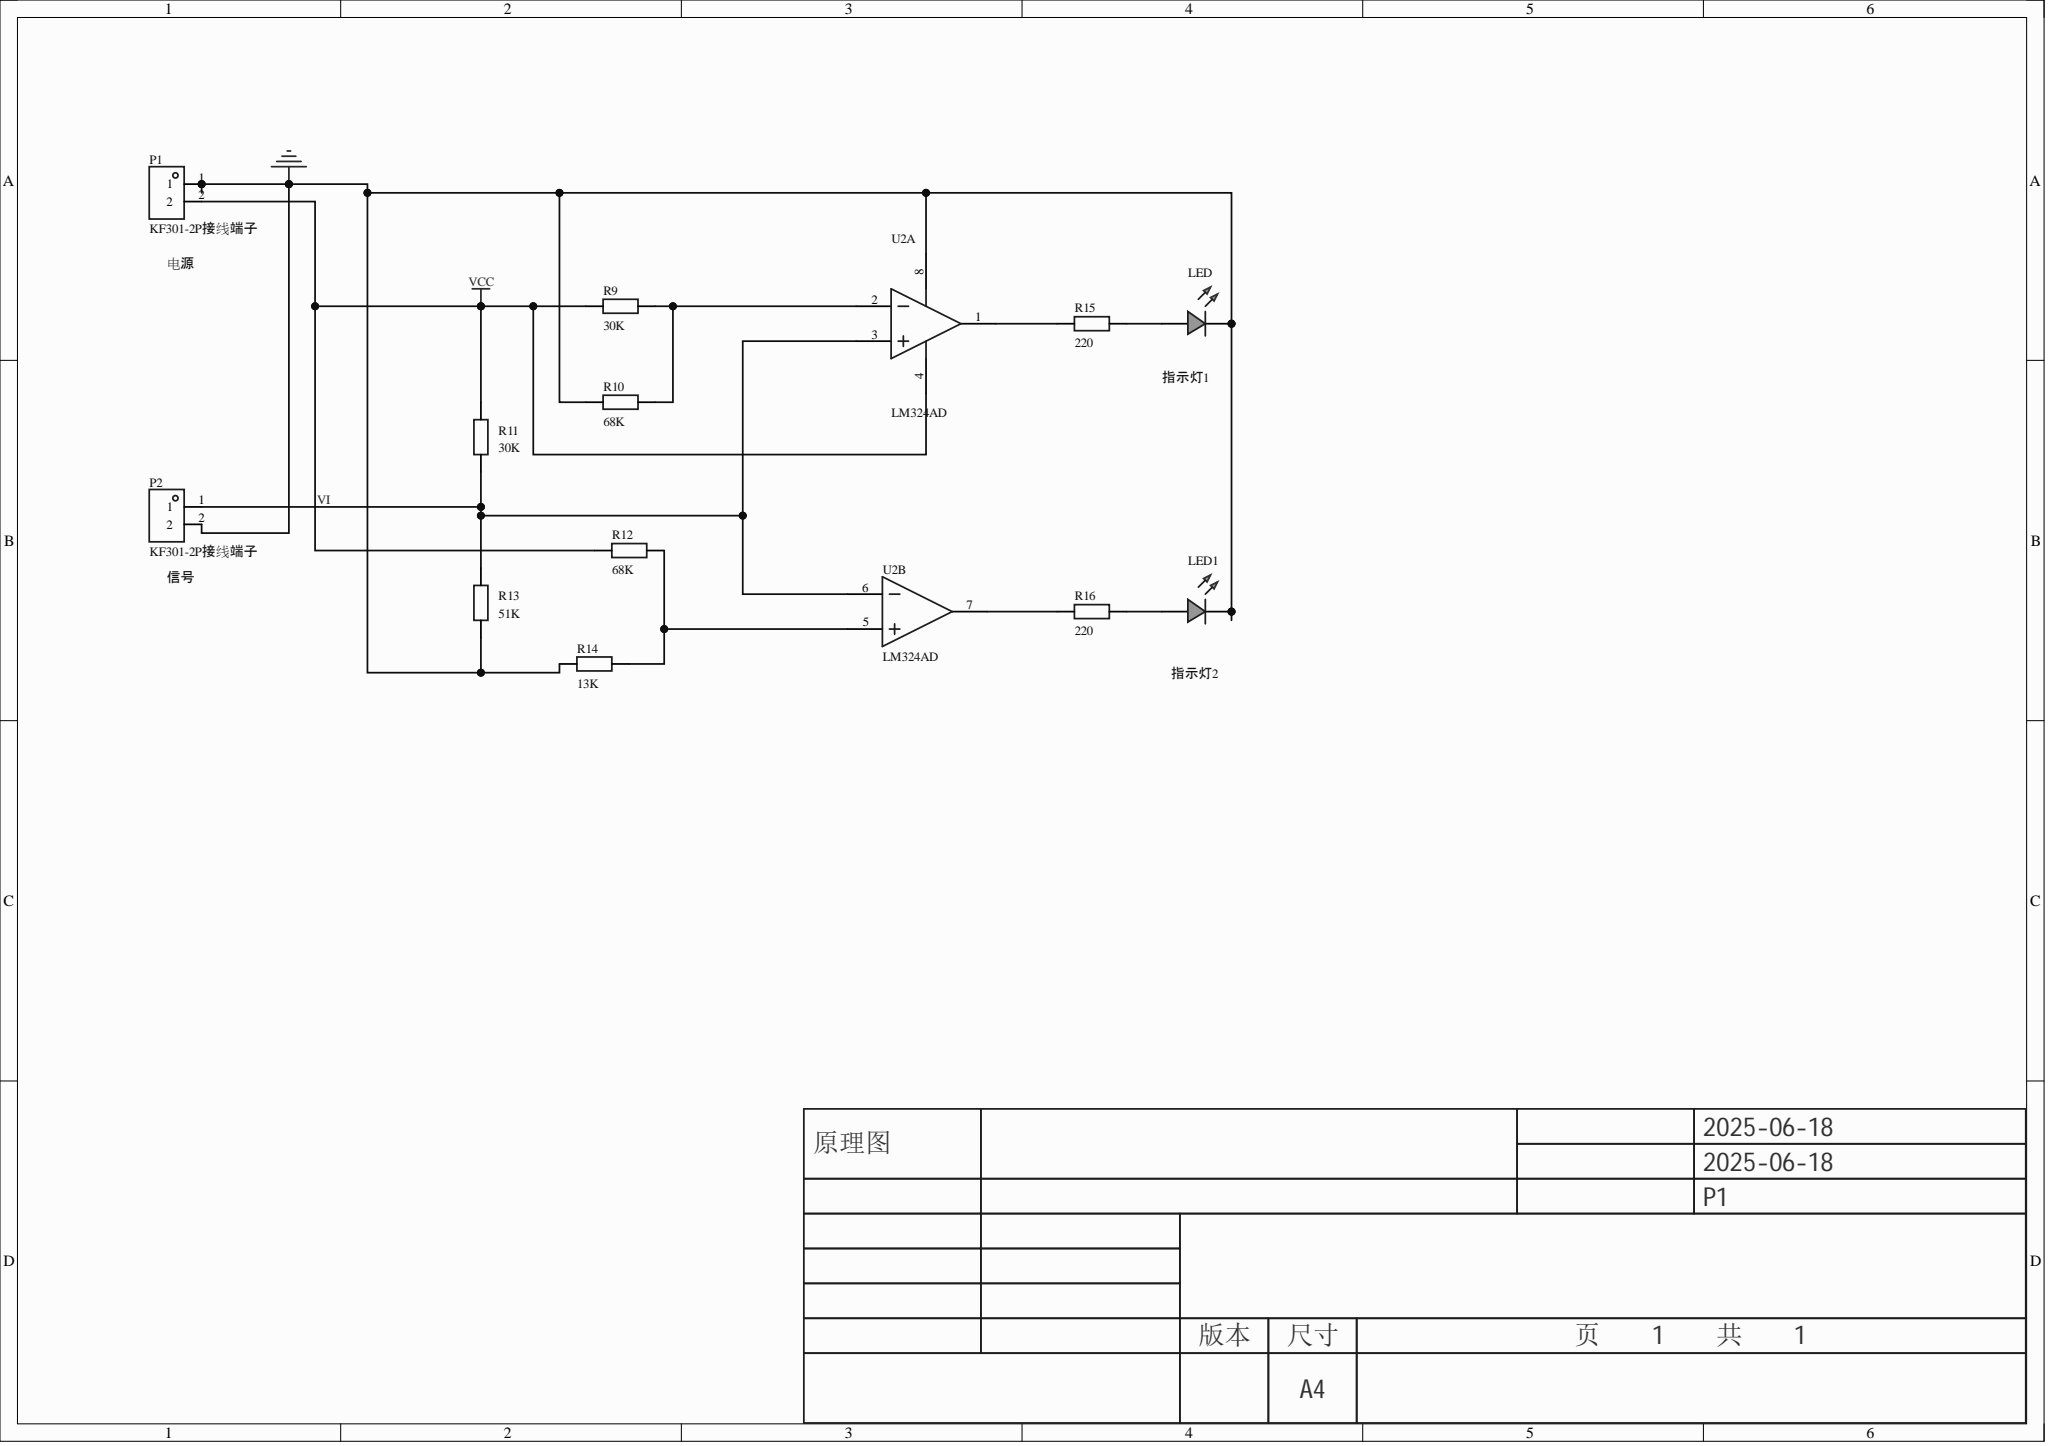Circuit board | Altium Designer | 13 parts | 9 nets
Bill of materials:
Comment,Description,Designator,Footprint,LibRef,Quantity
"","","LED, LED1","LED-TH_5mm","LED_TH-G_5mm","2"
"KF301-2P接线端子","","P1, P2","CONN-TH_XY301V-A-5.0-2P","KF301-2P接线端子","2"
"30K","","R9, R11","Res_1/8W","Res_AXIAL-1/8W","2"
"68K","","R10, R12","Res_1/8W","Res_AXIAL-1/8W","2"
"51K","","R13","Res_1/8W","Res_AXIAL-1/8W","1"
"13K","","R14","Res_1/8W","Res_AXIAL-1/8W","1"
"220","","R15, R16","Res_1/8W","Res_AXIAL-1/8W","2"
"LM324AD","放大器数:双路;轨到轨:-;增益带宽积(GBP):10MHz;输入失调电压(Vos):5mV;压摆率(SR):11V/us;输入偏置电流(Ib):500nA;","U2","DIP-8_L9.3-W6.4-P2.54-LS7.6-BL","NE5532N","1"
Netlist (Protel format):
[
LED
LED-TH_5mm




]
[
LED1
LED-TH_5mm




]
[
P1
CONN-TH_XY301V-A-5.0-2P
KF301-2P接线端子



]
[
P2
CONN-TH_XY301V-A-5.0-2P
KF301-2P接线端子



]
[
R9
Res_1/8W
30K



]
[
R10
Res_1/8W
68K



]
[
R11
Res_1/8W
30K



]
[
R12
Res_1/8W
68K



]
[
R13
Res_1/8W
51K



]
[
R14
Res_1/8W
13K



]
[
R15
Res_1/8W
220



]
[
R16
Res_1/8W
220



]
[
U2
DIP-8_L9.3-W6.4-P2.54-LS7.6-BL
LM324AD



]
(
VI
P2-1
R11-1
R13-2
U2-3
U2-6
)
(
VCC
P1-2
R9-1
R11-2
R12-1
U2-4
)
(
NetR16_1
R16-1
U2-7
)
(
NetR15_1
R15-1
U2-1
)
(
NetR12_2
R12-2
R14-2
U2-5
)
(
NetR9_2
R9-2
R10-2
U2-2
)
(
NetLED_1
LED-1
R15-2
)
(
NetLED1_1
LED1-1
R16-2
)
(
GND
LED-2
LED1-2
P1-1
P2-2
R10-1
R13-1
R14-1
U2-8
)